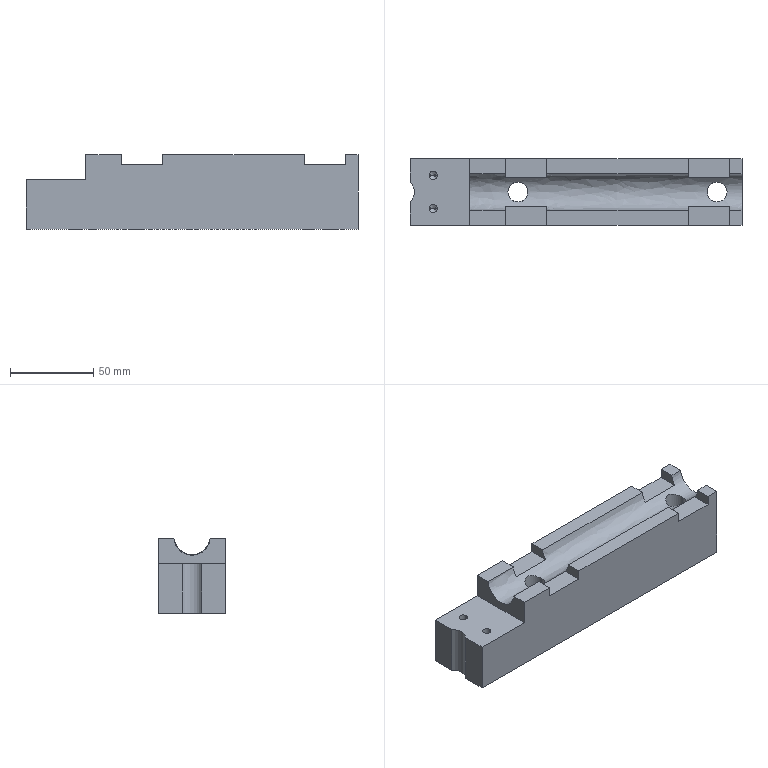NC program | NX | posted with a generic post
Lines 21106 to 21908 of 104568:
(FIXED_CONTOUR_COPY , TOOL : R3)
N42192 T08 M6
N42194 G54
N42196 G17 G0 G90 X-64.582 Y7.713 S9500 M3
N42198 G43 Z30. H8
N42200 Z2.4
N42202 G94 G1 Z-3.445 F500.
N42204 G3 X-64.003 Y7.869 R0.6
N42206 G1 X-63.992 Y7.88 Z-3.384 F3500.
N42208 X-63.931 Y7.94 Z-2.963
N42210 X-63.902 Y7.969 Z-2.719
N42212 X-63.865 Z-2.715
N42214 X-63.894 Y7.94 Z-2.959
N42216 X-63.955 Y7.88 Z-3.381
N42218 X-64.001 Y7.833 Z-3.636
N42220 Y7.819 Z-3.708
N42222 X-64. Y7.791 Z-3.825
N42224 X-63.971 Y7.819 Z-3.706
N42226 X-63.911 Y7.88 Z-3.378
N42228 X-63.85 Y7.94 Z-2.955
N42230 X-63.821 Y7.97 Z-2.712
N42232 X-63.776 Y7.969 Z-2.711
N42234 X-63.805 Y7.94 Z-2.95
N42236 X-63.866 Y7.88 Z-3.375
N42238 X-63.926 Y7.819 Z-3.704
N42240 X-63.999 Y7.747 Z-4.004
N42242 X-63.998 Y7.706 Z-4.172
N42244 X-63.884 Y7.819 Z-3.702
N42246 X-63.824 Y7.88 Z-3.372
N42248 X-63.763 Y7.94 Z-2.945
N42250 X-63.734 Y7.969 Z-2.711
N42252 X-63.69
N42254 X-63.719 Y7.94 Z-2.94
N42256 X-63.779 Y7.88 Z-3.369
N42258 X-63.839 Y7.819 Z-3.7
N42260 X-63.96 Y7.699 Z-4.201
N42262 X-63.997 Y7.662 Z-4.326
N42264 Y7.613 Z-4.49
N42266 X-63.911 Y7.699 Z-4.201
N42268 X-63.79 Y7.819 Z-3.697
N42270 X-63.73 Y7.88 Z-3.366
N42272 X-63.669 Y7.94 Z-2.936
N42274 X-63.641 Y7.969 Z-2.711
N42276 X-63.584 Z-2.71
N42278 X-63.62 Y7.932 Z-2.993
N42280 X-63.673 Y7.88 Z-3.363
N42282 X-63.733 Y7.819 Z-3.695
N42284 X-63.854 Y7.699 Z-4.201
N42286 X-63.903 Y7.649 Z-4.364
N42288 X-63.975 Y7.578 Z-4.608
N42290 X-63.996 Y7.556 Z-4.669
N42292 X-63.997 Y7.496 Z-4.833
N42294 X-63.915 Y7.578 Z-4.606
N42296 X-63.839 Y7.654 Z-4.349
N42298 X-63.794 Y7.699 Z-4.202
N42300 X-63.673 Y7.819 Z-3.692
N42302 X-63.613 Y7.88 Z-3.363
N42304 X-63.552 Y7.94 Z-2.93
N42306 X-63.524 Y7.968 Z-2.71
N42308 X-63.463
N42310 X-63.512 Y7.919 Z-3.087
N42312 X-63.551 Y7.88 Z-3.362
N42314 X-63.611 Y7.819 Z-3.692
N42316 X-63.732 Y7.699 Z-4.202
N42318 X-63.811 Y7.619 Z-4.463
N42320 X-63.853 Y7.578 Z-4.604
N42322 X-63.973 Y7.457 Z-4.94
N42324 X-63.997 Y7.433 Z-4.997
N42326 X-63.998 Y7.363 Z-5.165
N42328 X-63.903 Y7.457 Z-4.937
N42330 X-63.783 Y7.578 Z-4.602
N42332 X-63.662 Y7.699 Z-4.202
N42334 X-63.541 Y7.819 Z-3.691
N42336 X-63.481 Y7.88 Z-3.362
N42338 X-63.42 Y7.94 Z-2.924
N42340 X-63.393 Y7.968 Z-2.709
N42342 X-63.324
N42344 X-63.388 Y7.904 Z-3.195
N42346 X-63.411 Y7.88 Z-3.362
N42348 X-63.472 Y7.819 Z-3.691
N42350 X-63.593 Y7.699 Z-4.202
N42352 X-63.714 Y7.578 Z-4.6
N42354 X-63.834 Y7.457 Z-4.935
N42356 X-63.955 Y7.336 Z-5.226
N42358 X-63.999 Y7.293 Z-5.32
N42360 Y7.223 Z-5.468
N42362 X-63.886 Y7.336 Z-5.225
N42364 X-63.766 Y7.457 Z-4.933
N42366 X-63.645 Y7.578 Z-4.598
N42368 X-63.524 Y7.699 Z-4.203
N42370 X-63.403 Y7.819 Z-3.69
N42372 X-63.343 Y7.88 Z-3.361
N42374 X-63.255 Y7.968 Z-2.708
N42376 X-63.18 Y7.967
N42378 X-63.268 Y7.88 Z-3.361
N42380 X-63.328 Y7.819 Z-3.69
N42382 X-63.449 Y7.699 Z-4.203
N42384 X-63.57 Y7.578 Z-4.598
N42386 X-63.69 Y7.457 Z-4.93
N42388 X-63.811 Y7.336 Z-5.223
N42390 X-63.932 Y7.215 Z-5.483
N42392 X-64. Y7.148 Z-5.612
N42394 X-64.001 Y7.064 Z-5.768
N42396 X-63.85 Y7.215 Z-5.481
N42398 X-63.72 Y7.345 Z-5.2
N42400 X-63.608 Y7.457 Z-4.93
N42402 X-63.487 Y7.578 Z-4.596
N42404 X-63.366 Y7.699 Z-4.203
N42406 X-63.246 Y7.819 Z-3.689
N42408 X-63.185 Y7.88 Z-3.36
N42410 X-63.098 Y7.967 Z-2.707
N42412 X-63.02
N42414 X-63.107 Y7.88 Z-3.36
N42416 X-63.167 Y7.819 Z-3.689
N42418 X-63.288 Y7.699 Z-4.203
N42420 X-63.409 Y7.578 Z-4.595
N42422 X-63.53 Y7.457 Z-4.929
N42424 X-63.65 Y7.336 Z-5.22
N42426 X-63.771 Y7.215 Z-5.479
N42428 X-64.001 Y6.986 Z-5.915
N42430 Y6.904 Z-6.052
N42432 X-63.931 Y6.974 Z-5.936
N42434 X-63.689 Y7.216 Z-5.477
N42436 X-63.569 Y7.336 Z-5.219
N42438 X-63.448 Y7.457 Z-4.928
N42440 X-63.327 Y7.578 Z-4.594
N42442 X-63.206 Y7.699 Z-4.203
N42444 X-63.086 Y7.819 Z-3.689
N42446 X-63.025 Y7.88 Z-3.359
N42448 X-62.939 Y7.966 Z-2.707
N42450 X-62.853
N42452 X-62.939 Y7.88 Z-3.358
N42454 X-63. Y7.819 Z-3.689
N42456 X-63.12 Y7.699 Z-4.204
N42458 X-63.241 Y7.578 Z-4.593
N42460 X-63.362 Y7.457 Z-4.927
N42462 X-63.483 Y7.336 Z-5.219
N42464 X-63.604 Y7.215 Z-5.477
N42466 X-63.845 Y6.974 Z-5.934
N42468 X-64.002 Y6.817 Z-6.193
N42470 Y6.728 Z-6.338
N42472 X-63.756 Y6.974 Z-5.932
N42474 X-63.515 Y7.215 Z-5.477
N42476 X-63.394 Y7.336 Z-5.218
N42478 X-63.273 Y7.457 Z-4.926
N42480 X-63.152 Y7.578 Z-4.593
N42482 X-63.031 Y7.699 Z-4.204
N42484 X-62.911 Y7.819 Z-3.689
N42486 X-62.85 Y7.88 Z-3.357
N42488 X-62.764 Y7.966 Z-2.707
N42490 X-62.674
N42492 X-62.76 Y7.88 Z-3.356
N42494 X-62.82 Y7.819 Z-3.689
N42496 X-62.941 Y7.699 Z-4.205
N42498 X-63.062 Y7.578 Z-4.593
N42500 X-63.182 Y7.457 Z-4.925
N42502 X-63.303 Y7.336 Z-5.218
N42504 X-63.424 Y7.215 Z-5.476
N42506 X-63.666 Y6.974 Z-5.931
N42508 X-63.907 Y6.732 Z-6.33
N42510 X-64.002 Y6.638 Z-6.472
N42512 X-64.001 Y6.546 Z-6.608
N42514 X-63.815 Y6.732 Z-6.328
N42516 X-63.573 Y6.974 Z-5.93
N42518 X-63.332 Y7.215 Z-5.476
N42520 X-63.211 Y7.336 Z-5.218
N42522 X-63.09 Y7.457 Z-4.925
N42524 X-62.969 Y7.578 Z-4.593
N42526 X-62.848 Y7.699 Z-4.205
N42528 X-62.728 Y7.819 Z-3.689
N42530 X-62.667 Y7.88 Z-3.356
N42532 X-62.582 Y7.965 Z-2.707
N42534 X-62.485
N42536 X-62.532 Y7.919 Z-3.06
N42538 X-62.57 Y7.88 Z-3.356
N42540 X-62.631 Y7.819 Z-3.689
N42542 X-62.751 Y7.699 Z-4.206
N42544 X-62.872 Y7.578 Z-4.593
N42546 X-62.993 Y7.457 Z-4.926
N42548 X-63.114 Y7.336 Z-5.217
N42550 X-63.235 Y7.215 Z-5.476
N42552 X-63.476 Y6.974 Z-5.929
N42554 X-63.718 Y6.732 Z-6.327
N42556 X-63.96 Y6.491 Z-6.689
N42558 X-64.001 Y6.449 Z-6.745
N42560 Y6.352 Z-6.874
N42562 X-63.862 Y6.491 Z-6.687
N42564 X-63.621 Y6.732 Z-6.326
N42566 X-63.379 Y6.974 Z-5.929
N42568 X-63.138 Y7.215 Z-5.475
N42570 X-63.017 Y7.336 Z-5.217
N42572 X-62.896 Y7.457 Z-4.926
N42574 X-62.775 Y7.578 Z-4.594
N42576 X-62.654 Y7.699 Z-4.207
N42578 X-62.534 Y7.819 Z-3.689
N42580 X-62.473 Y7.88 Z-3.356
N42582 X-62.413 Y7.94 Z-2.885
N42584 X-62.389 Y7.965 Z-2.708
N42586 X-62.295 Y7.964
N42588 X-62.319 Y7.94 Z-2.882
N42590 X-62.379 Y7.88 Z-3.356
N42592 X-62.44 Y7.819 Z-3.69
N42594 X-62.561 Y7.699 Z-4.207
N42596 X-62.681 Y7.578 Z-4.594
N42598 X-62.802 Y7.457 Z-4.926
N42600 X-62.923 Y7.336 Z-5.218
N42602 X-63.044 Y7.215 Z-5.476
N42604 X-63.285 Y6.974 Z-5.928
N42606 X-63.527 Y6.732 Z-6.326
N42608 X-63.769 Y6.491 Z-6.685
N42610 X-64. Y6.259 Z-6.999
N42612 Y6.163 Z-7.116
N42614 X-63.914 Y6.249 Z-7.011
N42616 X-63.672 Y6.491 Z-6.684
N42618 X-63.43 Y6.732 Z-6.326
N42620 X-63.189 Y6.974 Z-5.928
N42622 X-62.947 Y7.215 Z-5.476
N42624 X-62.826 Y7.336 Z-5.218
N42626 X-62.705 Y7.458 Z-4.924
N42628 X-62.585 Y7.578 Z-4.595
N42630 X-62.464 Y7.699 Z-4.208
N42632 X-62.343 Y7.819 Z-3.69
N42634 X-62.283 Y7.88 Z-3.356
N42636 X-62.222 Y7.941 Z-2.876
N42638 X-62.199 Y7.964 Z-2.708
N42640 X-62.099
N42642 X-62.133 Y7.93 Z-2.962
N42644 X-62.183 Y7.88 Z-3.356
N42646 X-62.243 Y7.819 Z-3.691
N42648 X-62.364 Y7.699 Z-4.209
N42650 X-62.485 Y7.578 Z-4.596
N42652 X-62.605 Y7.457 Z-4.927
N42654 X-62.726 Y7.336 Z-5.218
N42656 X-62.847 Y7.215 Z-5.476
N42658 X-63.089 Y6.974 Z-5.928
N42660 X-63.33 Y6.732 Z-6.325
N42662 X-63.572 Y6.491 Z-6.684
N42664 X-63.813 Y6.249 Z-7.009
N42666 X-64. Y6.062 Z-7.236
N42668 Y6.007 Z-7.302
N42670 Y5.961 Z-7.351
N42672 X-63.954 Y6.007 Z-7.301
N42674 X-63.712 Y6.249 Z-7.007
N42676 X-63.471 Y6.491 Z-6.684
N42678 X-63.229 Y6.732 Z-6.325
N42680 X-62.988 Y6.974 Z-5.928
N42682 X-62.746 Y7.215 Z-5.476
N42684 X-62.625 Y7.336 Z-5.218
N42686 X-62.504 Y7.457 Z-4.927
N42688 X-62.384 Y7.578 Z-4.597
N42690 X-62.263 Y7.699 Z-4.21
N42692 X-62.142 Y7.819 Z-3.691
N42694 X-62.082 Y7.88 Z-3.355
N42696 X-62.021 Y7.94 Z-2.874
N42698 X-61.998 Y7.963 Z-2.709
N42700 X-61.898
N42702 X-61.92 Y7.94 Z-2.871
N42704 X-61.981 Y7.88 Z-3.354
N42706 X-62.041 Y7.819 Z-3.691
N42708 X-62.162 Y7.699 Z-4.21
N42710 X-62.283 Y7.578 Z-4.598
N42712 X-62.404 Y7.457 Z-4.928
N42714 X-62.524 Y7.336 Z-5.218
N42716 X-62.645 Y7.215 Z-5.476
N42718 X-62.887 Y6.974 Z-5.928
N42720 X-63.128 Y6.732 Z-6.325
N42722 X-63.37 Y6.491 Z-6.684
N42724 X-63.612 Y6.249 Z-7.007
N42726 X-63.853 Y6.007 Z-7.299
N42728 X-64. Y5.861 Z-7.459
N42730 Y5.76 Z-7.568
N42732 X-63.752 Y6.007 Z-7.298
N42734 X-63.511 Y6.249 Z-7.007
N42736 X-63.269 Y6.491 Z-6.684
N42738 X-63.027 Y6.732 Z-6.325
N42740 X-62.786 Y6.974 Z-5.928
N42742 X-62.544 Y7.215 Z-5.476
N42744 X-62.423 Y7.336 Z-5.218
N42746 X-62.303 Y7.457 Z-4.928
N42748 X-62.182 Y7.578 Z-4.599
N42750 X-62.061 Y7.699 Z-4.211
N42752 X-61.94 Y7.819 Z-3.692
N42754 X-61.88 Y7.88 Z-3.353
N42756 X-61.809 Y7.95 Z-2.797
N42758 X-61.797 Y7.963 Z-2.709
N42760 X-61.696 Y7.962
N42762 X-61.719 Y7.94 Z-2.866
N42764 X-61.779 Y7.88 Z-3.352
N42766 X-61.839 Y7.819 Z-3.692
N42768 X-61.96 Y7.699 Z-4.212
N42770 X-62.081 Y7.578 Z-4.6
N42772 X-62.202 Y7.457 Z-4.929
N42774 X-62.323 Y7.336 Z-5.219
N42776 X-62.443 Y7.215 Z-5.477
N42778 X-62.685 Y6.974 Z-5.927
N42780 X-62.927 Y6.732 Z-6.325
N42782 X-63.168 Y6.491 Z-6.684
N42784 X-63.41 Y6.249 Z-7.006
N42786 X-63.651 Y6.007 Z-7.297
N42788 X-63.893 Y5.766 Z-7.56
N42790 X-64. Y5.659 Z-7.668
N42792 Y5.558 Z-7.768
N42794 X-63.792 Y5.766 Z-7.559
N42796 X-63.551 Y6.007 Z-7.297
N42798 X-63.309 Y6.249 Z-7.006
N42800 X-63.067 Y6.491 Z-6.684
N42802 X-62.826 Y6.732 Z-6.325
N42804 X-62.584 Y6.974 Z-5.927
N42806 X-62.343 Y7.215 Z-5.477
N42808 X-62.222 Y7.336 Z-5.219
N42810 X-62.101 Y7.457 Z-4.93
N42812 X-61.98 Y7.578 Z-4.601
N42814 X-61.859 Y7.699 Z-4.213
N42816 X-61.739 Y7.819 Z-3.693
N42818 X-61.678 Y7.88 Z-3.352
N42820 X-61.618 Y7.94 Z-2.866
N42822 X-61.596 Y7.962 Z-2.71
N42824 X-61.495
N42826 X-61.517 Y7.94 Z-2.866
N42828 X-61.577 Y7.88 Z-3.351
N42830 X-61.638 Y7.819 Z-3.693
N42832 X-61.759 Y7.699 Z-4.214
N42834 X-61.879 Y7.578 Z-4.602
N42836 X-62. Y7.457 Z-4.93
N42838 X-62.121 Y7.336 Z-5.219
N42840 X-62.242 Y7.215 Z-5.477
N42842 X-62.484 Y6.974 Z-5.927
N42844 X-62.725 Y6.732 Z-6.325
N42846 X-62.967 Y6.491 Z-6.684
N42848 X-63.208 Y6.249 Z-7.006
N42850 X-63.45 Y6.007 Z-7.297
N42852 X-63.692 Y5.766 Z-7.557
N42854 X-63.933 Y5.524 Z-7.8
N42856 X-64. Y5.457 Z-7.862
N42858 Y5.357 Z-7.954
N42860 X-63.832 Y5.524 Z-7.799
N42862 X-63.591 Y5.766 Z-7.557
N42864 X-63.349 Y6.007 Z-7.297
N42866 X-63.108 Y6.249 Z-7.006
N42868 X-62.866 Y6.491 Z-6.684
N42870 X-62.624 Y6.732 Z-6.325
N42872 X-62.383 Y6.974 Z-5.927
N42874 X-62.141 Y7.215 Z-5.477
N42876 X-62.02 Y7.336 Z-5.218
N42878 X-61.9 Y7.457 Z-4.931
N42880 X-61.779 Y7.578 Z-4.603
N42882 X-61.658 Y7.699 Z-4.214
N42884 X-61.537 Y7.819 Z-3.694
N42886 X-61.477 Y7.88 Z-3.35
N42888 X-61.416 Y7.94 Z-2.867
N42890 X-61.394 Y7.962 Z-2.71
N42892 X-61.294 Z-2.711
N42894 X-61.326 Y7.93 Z-2.952
N42896 X-61.376 Y7.88 Z-3.349
N42898 X-61.436 Y7.819 Z-3.694
N42900 X-61.557 Y7.699 Z-4.215
N42902 X-61.678 Y7.578 Z-4.604
N42904 X-61.799 Y7.457 Z-4.931
N42906 X-61.92 Y7.336 Z-5.218
N42908 X-62.04 Y7.215 Z-5.477
N42910 X-62.282 Y6.974 Z-5.927
N42912 X-62.524 Y6.732 Z-6.324
N42914 X-62.765 Y6.491 Z-6.684
N42916 X-63.007 Y6.249 Z-7.006
N42918 X-63.248 Y6.007 Z-7.297
N42920 X-63.49 Y5.766 Z-7.557
N42922 X-63.732 Y5.524 Z-7.798
N42924 X-63.973 Y5.283 Z-8.021
N42926 X-64. Y5.256 Z-8.044
N42928 Y5.155 Z-8.129
N42930 X-63.872 Y5.283 Z-8.02
N42932 X-63.631 Y5.524 Z-7.797
N42934 X-63.389 Y5.766 Z-7.557
N42936 X-63.148 Y6.007 Z-7.297
N42938 X-62.906 Y6.249 Z-7.006
N42940 X-62.664 Y6.491 Z-6.684
N42942 X-62.423 Y6.732 Z-6.324
N42944 X-62.181 Y6.974 Z-5.927
N42946 X-61.94 Y7.215 Z-5.477
N42948 X-61.819 Y7.336 Z-5.218
N42950 X-61.698 Y7.457 Z-4.932
N42952 X-61.577 Y7.578 Z-4.605
N42954 X-61.456 Y7.699 Z-4.216
N42956 X-61.336 Y7.819 Z-3.695
N42958 X-61.275 Y7.88 Z-3.348
N42960 X-61.215 Y7.94 Z-2.867
N42962 X-61.193 Y7.962 Z-2.711
N42964 X-61.093
N42966 X-61.114 Y7.94 Z-2.868
N42968 X-61.174 Y7.88 Z-3.347
N42970 X-61.235 Y7.819 Z-3.695
N42972 X-61.356 Y7.699 Z-4.217
N42974 X-61.476 Y7.578 Z-4.606
N42976 X-61.597 Y7.457 Z-4.933
N42978 X-61.718 Y7.336 Z-5.218
N42980 X-61.839 Y7.215 Z-5.477
N42982 X-62.08 Y6.974 Z-5.927
N42984 X-62.322 Y6.732 Z-6.324
N42986 X-62.564 Y6.491 Z-6.684
N42988 X-62.805 Y6.249 Z-7.006
N42990 X-63.047 Y6.007 Z-7.297
N42992 X-63.289 Y5.766 Z-7.557
N42994 X-63.53 Y5.524 Z-7.797
N42996 X-63.772 Y5.283 Z-8.018
N42998 X-64. Y5.054 Z-8.214
N43000 Y4.953 Z-8.294
N43002 X-63.913 Y5.041 Z-8.224
N43004 X-63.671 Y5.283 Z-8.017
N43006 X-63.429 Y5.524 Z-7.797
N43008 X-63.188 Y5.766 Z-7.557
N43010 X-62.946 Y6.007 Z-7.297
N43012 X-62.705 Y6.249 Z-7.005
N43014 X-62.463 Y6.491 Z-6.684
N43016 X-62.221 Y6.732 Z-6.324
N43018 X-61.98 Y6.974 Z-5.926
N43020 X-61.738 Y7.215 Z-5.478
N43022 X-61.617 Y7.336 Z-5.218
N43024 X-61.497 Y7.457 Z-4.933
N43026 X-61.376 Y7.578 Z-4.607
N43028 X-61.255 Y7.699 Z-4.218
N43030 X-61.134 Y7.819 Z-3.695
N43032 X-61.074 Y7.88 Z-3.346
N43034 X-61.013 Y7.94 Z-2.869
N43036 X-60.992 Y7.962 Z-2.711
N43038 X-60.891 Z-2.712
N43040 X-60.936 Y7.917 Z-3.051
N43042 X-60.973 Y7.88 Z-3.345
N43044 X-61.034 Y7.819 Z-3.696
N43046 X-61.154 Y7.699 Z-4.218
N43048 X-61.275 Y7.578 Z-4.608
N43050 X-61.396 Y7.457 Z-4.934
N43052 X-61.517 Y7.336 Z-5.217
N43054 X-61.638 Y7.215 Z-5.477
N43056 X-61.879 Y6.974 Z-5.926
N43058 X-62.121 Y6.732 Z-6.324
N43060 X-62.362 Y6.491 Z-6.684
N43062 X-62.604 Y6.249 Z-7.005
N43064 X-62.846 Y6.007 Z-7.297
N43066 X-63.087 Y5.766 Z-7.557
N43068 X-63.329 Y5.524 Z-7.797
N43070 X-63.57 Y5.283 Z-8.017
N43072 X-63.812 Y5.041 Z-8.223
N43074 X-64. Y4.853 Z-8.372
N43076 Y4.752 Z-8.448
N43078 X-63.953 Y4.799 Z-8.413
N43080 X-63.686 Y5.067 Z-8.199
N43082 X-63.47 Y5.283 Z-8.017
N43084 X-63.228 Y5.524 Z-7.797
N43086 X-62.987 Y5.766 Z-7.557
N43088 X-62.745 Y6.007 Z-7.297
N43090 X-62.503 Y6.249 Z-7.005
N43092 X-62.262 Y6.491 Z-6.684
N43094 X-62.02 Y6.732 Z-6.324
N43096 X-61.779 Y6.974 Z-5.926
N43098 X-61.537 Y7.215 Z-5.477
N43100 X-61.416 Y7.336 Z-5.217
N43102 X-61.295 Y7.457 Z-4.934
N43104 X-61.175 Y7.578 Z-4.609
N43106 X-61.054 Y7.699 Z-4.219
N43108 X-60.933 Y7.819 Z-3.696
N43110 X-60.873 Y7.88 Z-3.344
N43112 X-60.812 Y7.94 Z-2.871
N43114 X-60.79 Y7.962 Z-2.712
N43116 X-60.69
N43118 X-60.711 Y7.94 Z-2.871
N43120 X-60.772 Y7.88 Z-3.343
N43122 X-60.832 Y7.819 Z-3.696
N43124 X-60.953 Y7.699 Z-4.219
N43126 X-61.074 Y7.578 Z-4.61
N43128 X-61.194 Y7.457 Z-4.935
N43130 X-61.315 Y7.336 Z-5.217
N43132 X-61.436 Y7.215 Z-5.477
N43134 X-61.678 Y6.974 Z-5.926
N43136 X-61.919 Y6.732 Z-6.323
N43138 X-62.161 Y6.491 Z-6.684
N43140 X-62.403 Y6.249 Z-7.005
N43142 X-62.644 Y6.007 Z-7.297
N43144 X-62.886 Y5.766 Z-7.557
N43146 X-63.127 Y5.524 Z-7.797
N43148 X-63.369 Y5.283 Z-8.017
N43150 X-63.611 Y5.041 Z-8.221
N43152 X-63.852 Y4.799 Z-8.412
N43154 X-64. Y4.651 Z-8.52
N43156 Y4.55 Z-8.592
N43158 X-63.751 Y4.799 Z-8.411
N43160 X-63.51 Y5.041 Z-8.221
N43162 X-63.268 Y5.283 Z-8.017
N43164 X-63.026 Y5.524 Z-7.796
N43166 X-62.785 Y5.766 Z-7.557
N43168 X-62.543 Y6.007 Z-7.297
N43170 X-62.302 Y6.249 Z-7.005
N43172 X-62.06 Y6.491 Z-6.684
N43174 X-61.818 Y6.732 Z-6.323
N43176 X-61.577 Y6.974 Z-5.925
N43178 X-61.335 Y7.215 Z-5.477
N43180 X-61.206 Y7.345 Z-5.198
N43182 X-61.094 Y7.457 Z-4.936
N43184 X-60.973 Y7.578 Z-4.611
N43186 X-60.852 Y7.699 Z-4.22
N43188 X-60.731 Y7.819 Z-3.696
N43190 X-60.671 Y7.88 Z-3.342
N43192 X-60.61 Y7.94 Z-2.871
N43194 X-60.589 Y7.962 Z-2.713
N43196 X-60.488
N43198 X-60.509 Y7.94 Z-2.87
N43200 X-60.57 Y7.88 Z-3.341
N43202 X-60.63 Y7.819 Z-3.696
N43204 X-60.643 Y7.806 Z-3.759
N43206 X-60.751 Y7.699 Z-4.219
N43208 X-60.872 Y7.578 Z-4.612
N43210 X-60.993 Y7.457 Z-4.936
N43212 X-61.113 Y7.336 Z-5.217
N43214 X-61.234 Y7.215 Z-5.476
N43216 X-61.476 Y6.974 Z-5.925
N43218 X-61.717 Y6.732 Z-6.323
N43220 X-61.959 Y6.491 Z-6.684
N43222 X-62.201 Y6.249 Z-7.005
N43224 X-62.442 Y6.007 Z-7.297
N43226 X-62.684 Y5.766 Z-7.557
N43228 X-62.926 Y5.524 Z-7.796
N43230 X-63.167 Y5.283 Z-8.017
N43232 X-63.409 Y5.041 Z-8.221
N43234 X-63.65 Y4.799 Z-8.41
N43236 X-63.892 Y4.558 Z-8.586
N43238 X-64. Y4.449 Z-8.659
N43240 Y4.349 Z-8.726
N43242 X-63.791 Y4.558 Z-8.585
N43244 X-63.549 Y4.799 Z-8.41
N43246 X-63.308 Y5.041 Z-8.221
N43248 X-63.066 Y5.283 Z-8.017
N43250 X-62.825 Y5.524 Z-7.796
N43252 X-62.583 Y5.766 Z-7.557
N43254 X-62.341 Y6.007 Z-7.297
N43256 X-62.1 Y6.249 Z-7.004
N43258 X-61.858 Y6.491 Z-6.684
N43260 X-61.617 Y6.732 Z-6.323
N43262 X-61.375 Y6.974 Z-5.925
N43264 X-61.133 Y7.215 Z-5.476
N43266 X-61.013 Y7.336 Z-5.217
N43268 X-60.892 Y7.457 Z-4.937
N43270 X-60.771 Y7.578 Z-4.613
N43272 X-60.65 Y7.699 Z-4.22
N43274 X-60.636 Y7.713 Z-4.164
N43276 X-60.554 Y7.795 Z-3.811
N43278 X-60.529 Y7.819 Z-3.696
N43280 X-60.469 Y7.88 Z-3.341
N43282 X-60.409 Y7.94 Z-2.869
N43284 X-60.387 Y7.962 Z-2.713
N43286 X-60.287 Y7.961 Z-2.714
N43288 X-60.308 Y7.94 Z-2.868
N43290 X-60.368 Y7.88 Z-3.34
N43292 X-60.428 Y7.819 Z-3.696
N43294 X-60.464 Y7.784 Z-3.864
N43296 X-60.521 Y7.727 Z-4.108
N43298 X-60.549 Y7.699 Z-4.22
N43300 X-60.67 Y7.578 Z-4.614
N43302 X-60.791 Y7.457 Z-4.938
N43304 X-60.912 Y7.336 Z-5.216
N43306 X-61.032 Y7.215 Z-5.476
N43308 X-61.274 Y6.974 Z-5.924
N43310 X-61.516 Y6.732 Z-6.322
N43312 X-61.757 Y6.491 Z-6.684
N43314 X-61.999 Y6.249 Z-7.004
N43316 X-62.24 Y6.007 Z-7.297
N43318 X-62.482 Y5.766 Z-7.557
N43320 X-62.724 Y5.524 Z-7.796
N43322 X-62.965 Y5.283 Z-8.016
N43324 X-63.207 Y5.041 Z-8.221
N43326 X-63.449 Y4.799 Z-8.41
N43328 X-63.689 Y4.559 Z-8.582
N43330 X-63.932 Y4.316 Z-8.747
N43332 X-64. Y4.248 Z-8.788
N43334 Y4.147 Z-8.848
N43336 X-63.831 Y4.316 Z-8.746
N43338 X-63.589 Y4.558 Z-8.583
N43340 X-63.348 Y4.799 Z-8.41
N43342 X-63.106 Y5.041 Z-8.221
N43344 X-62.864 Y5.283 Z-8.016
N43346 X-62.623 Y5.524 Z-7.796
N43348 X-62.381 Y5.766 Z-7.557
N43350 X-62.14 Y6.007 Z-7.297
N43352 X-61.898 Y6.249 Z-7.004
N43354 X-61.656 Y6.491 Z-6.684
N43356 X-61.415 Y6.732 Z-6.322
N43358 X-61.173 Y6.974 Z-5.924
N43360 X-60.932 Y7.215 Z-5.476
N43362 X-60.811 Y7.336 Z-5.216
N43364 X-60.69 Y7.457 Z-4.938
N43366 X-60.569 Y7.578 Z-4.614
N43368 X-60.448 Y7.699 Z-4.22
N43370 X-60.406 Y7.741 Z-4.052
N43372 X-60.374 Y7.773 Z-3.916
N43374 X-60.328 Y7.819 Z-3.696
N43376 X-60.267 Y7.88 Z-3.339
N43378 X-60.207 Y7.94 Z-2.867
N43380 X-60.186 Y7.961 Z-2.714
N43382 X-60.085
N43384 X-60.106 Y7.94 Z-2.866
N43386 X-60.166 Y7.88 Z-3.338
N43388 X-60.227 Y7.819 Z-3.696
N43390 X-60.291 Y7.756 Z-3.996
N43392 X-60.347 Y7.699 Z-4.22
N43394 X-60.468 Y7.578 Z-4.615
N43396 X-60.589 Y7.457 Z-4.939
N43398 X-60.71 Y7.336 Z-5.216
N43400 X-60.831 Y7.215 Z-5.475
N43402 X-61.072 Y6.974 Z-5.924
N43404 X-61.314 Y6.732 Z-6.322
N43406 X-61.555 Y6.491 Z-6.684
N43408 X-61.797 Y6.249 Z-7.004
N43410 X-62.039 Y6.007 Z-7.296
N43412 X-62.28 Y5.766 Z-7.557
N43414 X-62.522 Y5.524 Z-7.796
N43416 X-62.764 Y5.283 Z-8.016
N43418 X-63.005 Y5.041 Z-8.221
N43420 X-63.247 Y4.799 Z-8.409
N43422 X-63.488 Y4.558 Z-8.583
N43424 X-63.73 Y4.316 Z-8.745
N43426 X-64. Y4.046 Z-8.908
N43428 Y3.945 Z-8.968
N43430 X-63.629 Y4.316 Z-8.744
N43432 X-63.387 Y4.558 Z-8.583
N43434 X-63.146 Y4.799 Z-8.409
N43436 X-62.904 Y5.041 Z-8.221
N43438 X-62.663 Y5.283 Z-8.016
N43440 X-62.421 Y5.524 Z-7.796
N43442 X-62.179 Y5.766 Z-7.557
N43444 X-61.938 Y6.007 Z-7.296
N43446 X-61.696 Y6.249 Z-7.003
N43448 X-61.455 Y6.491 Z-6.684
N43450 X-61.213 Y6.732 Z-6.322
N43452 X-60.971 Y6.974 Z-5.923
N43454 X-60.73 Y7.215 Z-5.475
N43456 X-60.609 Y7.336 Z-5.216
N43458 X-60.488 Y7.457 Z-4.939
N43460 X-60.367 Y7.578 Z-4.615
N43462 X-60.247 Y7.699 Z-4.22
N43464 X-60.186 Y7.759 Z-3.982
N43466 X-60.126 Y7.819 Z-3.696
N43468 X-60.065 Y7.88 Z-3.338
N43470 X-60.005 Y7.94 Z-2.866
N43472 X-59.984 Y7.961 Z-2.714
N43474 X-59.884 Z-2.715
N43476 X-59.904 Y7.94 Z-2.865
N43478 X-59.964 Y7.88 Z-3.337
N43480 X-60.025 Y7.819 Z-3.697
N43482 X-60.085 Y7.759 Z-3.982
N43484 X-60.146 Y7.699 Z-4.22
N43486 X-60.267 Y7.578 Z-4.616
N43488 X-60.387 Y7.457 Z-4.939
N43490 X-60.508 Y7.336 Z-5.216
N43492 X-60.629 Y7.215 Z-5.474
N43494 X-60.871 Y6.974 Z-5.923
N43496 X-61.112 Y6.732 Z-6.322
N43498 X-61.354 Y6.491 Z-6.684
N43500 X-61.595 Y6.249 Z-7.003
N43502 X-61.837 Y6.007 Z-7.296
N43504 X-62.079 Y5.766 Z-7.557
N43506 X-62.32 Y5.524 Z-7.796
N43508 X-62.562 Y5.283 Z-8.016
N43510 X-62.803 Y5.041 Z-8.221
N43512 X-63.045 Y4.799 Z-8.409
N43514 X-63.287 Y4.558 Z-8.583
N43516 X-63.528 Y4.316 Z-8.744
N43518 X-64. Y3.844 Z-9.027
N43520 Y3.743 Z-9.079
N43522 X-63.911 Y3.833 Z-9.033
N43524 X-63.686 Y4.058 Z-8.897
N43526 X-63.427 Y4.316 Z-8.744
N43528 X-63.186 Y4.558 Z-8.583
N43530 X-62.944 Y4.799 Z-8.409
N43532 X-62.703 Y5.041 Z-8.221
N43534 X-62.461 Y5.283 Z-8.016
N43536 X-62.218 Y5.525 Z-7.794
N43538 X-61.978 Y5.766 Z-7.557
N43540 X-61.736 Y6.007 Z-7.296
N43542 X-61.494 Y6.249 Z-7.003
N43544 X-61.253 Y6.491 Z-6.684
N43546 X-61.011 Y6.732 Z-6.321
N43548 X-60.77 Y6.974 Z-5.923
N43550 X-60.528 Y7.215 Z-5.474
N43552 X-60.407 Y7.336 Z-5.216
N43554 X-60.286 Y7.457 Z-4.94
N43556 X-60.166 Y7.578 Z-4.616
N43558 X-60.045 Y7.699 Z-4.219
N43560 X-59.984 Y7.759 Z-3.983
N43562 X-59.924 Y7.819 Z-3.697
N43564 X-59.864 Y7.88 Z-3.337
N43566 X-59.803 Y7.94 Z-2.864
N43568 X-59.783 Y7.961 Z-2.715
N43570 X-59.682
N43572 X-59.702 Y7.94 Z-2.863
N43574 X-59.763 Y7.88 Z-3.336
N43576 X-59.823 Y7.819 Z-3.698
N43578 X-59.884 Y7.759 Z-3.983
N43580 X-59.944 Y7.699 Z-4.218
N43582 X-60.065 Y7.578 Z-4.616
N43584 X-60.186 Y7.457 Z-4.94
N43586 X-60.306 Y7.336 Z-5.216
N43588 X-60.427 Y7.215 Z-5.474
N43590 X-60.669 Y6.974 Z-5.923
N43592 X-60.91 Y6.732 Z-6.321
N43594 X-61.152 Y6.491 Z-6.684
N43596 X-61.394 Y6.249 Z-7.003
N43598 X-61.635 Y6.007 Z-7.296
N43600 X-61.877 Y5.766 Z-7.557
N43602 X-62.118 Y5.524 Z-7.795
N43604 X-62.36 Y5.283 Z-8.016
N43606 X-62.602 Y5.041 Z-8.221
N43608 X-62.843 Y4.799 Z-8.409
N43610 X-63.085 Y4.558 Z-8.584
N43612 X-63.326 Y4.316 Z-8.744
N43614 X-63.81 Y3.833 Z-9.032
N43616 X-64. Y3.642 Z-9.129
N43618 Y3.542 Z-9.18
N43620 X-63.709 Y3.833 Z-9.031
N43622 X-63.226 Y4.316 Z-8.744
N43624 X-62.984 Y4.558 Z-8.584
N43626 X-62.742 Y4.799 Z-8.409
N43628 X-62.501 Y5.041 Z-8.221
N43630 X-62.259 Y5.283 Z-8.016
N43632 X-62.018 Y5.524 Z-7.795
N43634 X-61.776 Y5.766 Z-7.557
N43636 X-61.534 Y6.007 Z-7.296
N43638 X-61.293 Y6.249 Z-7.003
N43640 X-61.051 Y6.491 Z-6.684
N43642 X-60.81 Y6.732 Z-6.321
N43644 X-60.568 Y6.974 Z-5.923
N43646 X-60.326 Y7.215 Z-5.473
N43648 X-60.206 Y7.336 Z-5.216
N43650 X-60.085 Y7.457 Z-4.939
N43652 X-59.964 Y7.578 Z-4.616
N43654 X-59.843 Y7.699 Z-4.217
N43656 X-59.783 Y7.759 Z-3.983
N43658 X-59.722 Y7.819 Z-3.698
N43660 X-59.662 Y7.88 Z-3.336
N43662 X-59.601 Y7.94 Z-2.862
N43664 X-59.581 Y7.96 Z-2.716
N43666 X-59.481
N43668 X-59.501 Y7.94 Z-2.861
N43670 X-59.561 Y7.88 Z-3.335
N43672 X-59.621 Y7.819 Z-3.698
N43674 X-59.682 Y7.759 Z-3.983
N43676 X-59.742 Y7.699 Z-4.217
N43678 X-59.863 Y7.578 Z-4.616
N43680 X-59.984 Y7.457 Z-4.939
N43682 X-60.105 Y7.336 Z-5.216
N43684 X-60.225 Y7.215 Z-5.473
N43686 X-60.467 Y6.974 Z-5.923
N43688 X-60.709 Y6.732 Z-6.321
N43690 X-60.95 Y6.491 Z-6.684
N43692 X-61.192 Y6.249 Z-7.002
N43694 X-61.433 Y6.007 Z-7.296
N43696 X-61.675 Y5.766 Z-7.557
N43698 X-61.917 Y5.524 Z-7.795
N43700 X-62.158 Y5.283 Z-8.016
N43702 X-62.4 Y5.041 Z-8.22
N43704 X-62.642 Y4.799 Z-8.409
N43706 X-62.883 Y4.558 Z-8.584
N43708 X-63.125 Y4.316 Z-8.744
N43710 X-63.608 Y3.833 Z-9.03
N43712 X-64. Y3.441 Z-9.23
N43714 Y3.34 Z-9.28
N43716 X-63.507 Y3.833 Z-9.03
N43718 X-63.024 Y4.316 Z-8.744
N43720 X-62.782 Y4.558 Z-8.584
N43722 X-62.541 Y4.799 Z-8.409
N43724 X-62.299 Y5.041 Z-8.22
N43726 X-62.057 Y5.283 Z-8.016
N43728 X-61.816 Y5.524 Z-7.795
N43730 X-61.574 Y5.766 Z-7.556
N43732 X-61.333 Y6.007 Z-7.296
N43734 X-61.091 Y6.249 Z-7.002
N43736 X-60.849 Y6.491 Z-6.684
N43738 X-60.608 Y6.732 Z-6.321
N43740 X-60.366 Y6.974 Z-5.922
N43742 X-60.125 Y7.215 Z-5.472
N43744 X-60.004 Y7.336 Z-5.216
N43746 X-59.883 Y7.457 Z-4.939
N43748 X-59.762 Y7.578 Z-4.616
N43750 X-59.641 Y7.699 Z-4.216
N43752 X-59.581 Y7.759 Z-3.983
N43754 X-59.521 Y7.819 Z-3.698
N43756 X-59.46 Y7.88 Z-3.335
N43758 X-59.4 Y7.94 Z-2.861
N43760 X-59.38 Y7.96 Z-2.716
N43762 X-59.279 Z-2.717
N43764 X-59.298 Y7.941 Z-2.853
N43766 X-59.359 Y7.88 Z-3.334
N43768 X-59.42 Y7.819 Z-3.698
N43770 X-59.48 Y7.759 Z-3.983
N43772 X-59.541 Y7.699 Z-4.215
N43774 X-59.661 Y7.578 Z-4.616
N43776 X-59.782 Y7.457 Z-4.939
N43778 X-59.903 Y7.336 Z-5.216
N43780 X-60.024 Y7.215 Z-5.471
N43782 X-60.265 Y6.974 Z-5.922
N43784 X-60.507 Y6.732 Z-6.321
N43786 X-60.749 Y6.491 Z-6.683
N43788 X-60.99 Y6.249 Z-7.002
N43790 X-61.232 Y6.007 Z-7.296